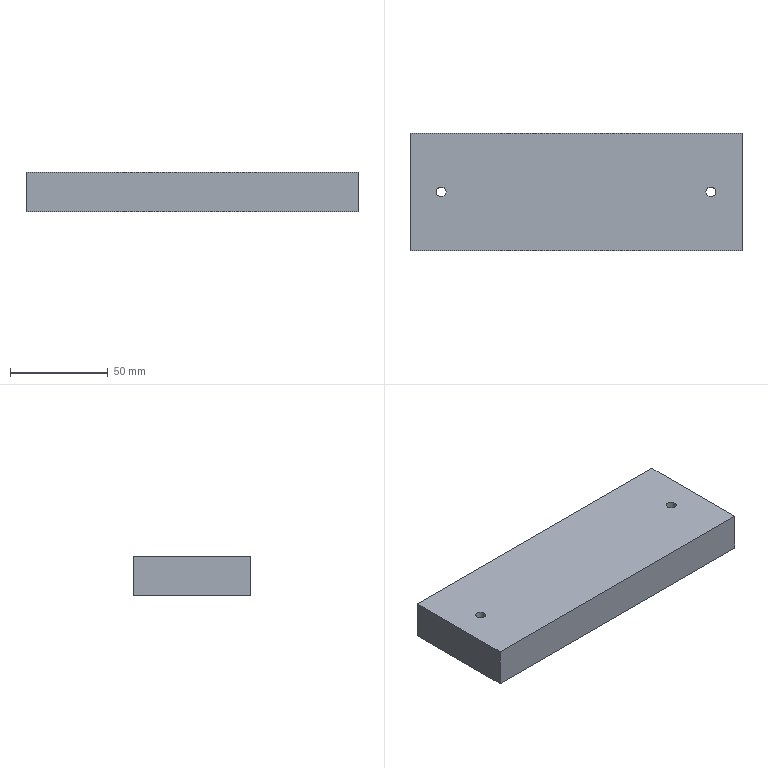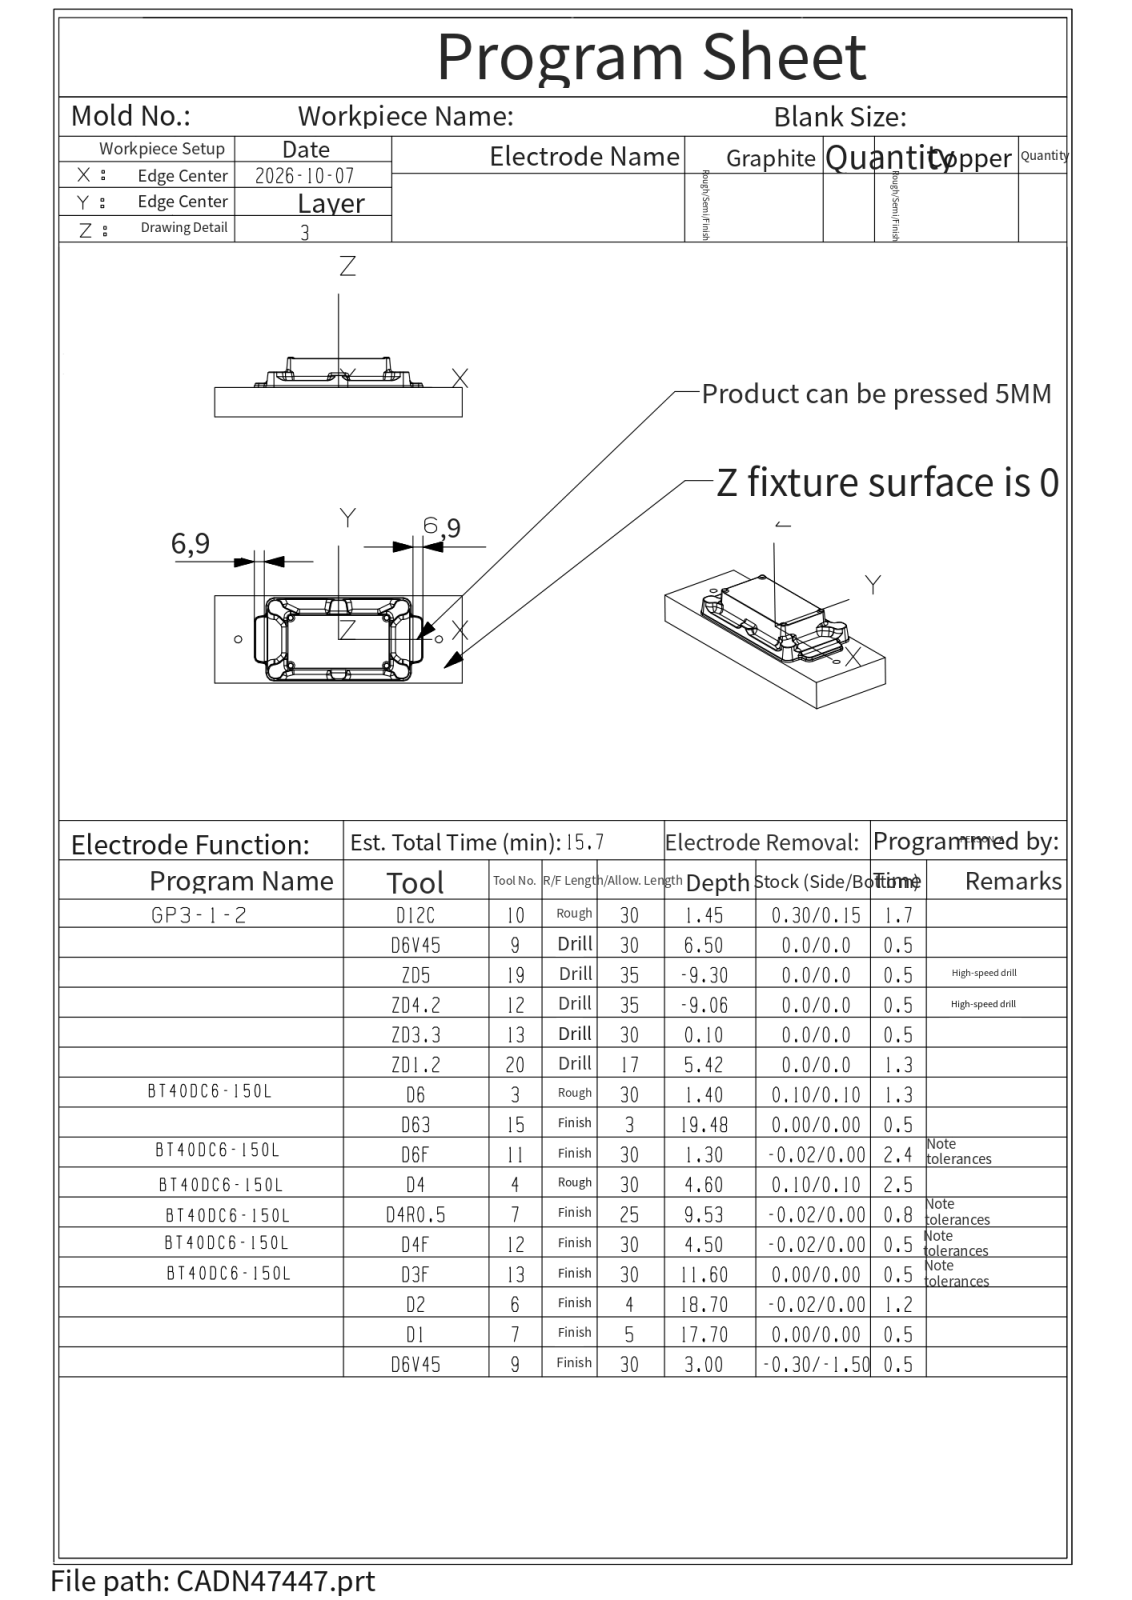NC program | NX | posted by the shop | part box 170 x 60 x 20 mm
Lines 1 to 1922 of 17682, first 1740 of 1922 lines:
%
O0001
G40 G49 G80 G90
G91 G28 Z0.0
N01
T10 M06
T02
( name=D12C    T=10 )
( XY = 0.30 )
( Z = 0.15 )
G00 G90 G54 X8.475 Y-8.751 S8000 M03
G43 Z27.98 H10 M08
Z23.088
G01 Z22.588 F4800.
X4.574 Y-7.625
G03 X-2.855 Y-11.725 I-1.664 J-5.765
G01 X-2.913 Y-11.927 F6000.
G02 X-3.047 Y-12.23 I-1.198 J.346
G01 X-3.202 Y-12.485
G02 X-3.859 Y-13.168 I-2.36 J1.613
X-5.449 Y-13.661 I-1.586 J2.307
X-6.373 Y-13.472 I.117 J2.913
X-7.504 Y-9.38 I.977 J2.472
X-5.57 Y-8.348 I2.111 J-1.627
X-3.795 Y-8.88 I.158 J-2.698
X-2.797 Y-11.523 I-1.611 J-2.118
G01 X-2.855 Y-11.725
G03 X1.245 Y-19.154 I5.765 J-1.664
G01 X5.151 Y-20.281
Z23.088
G00 Z24.48
G01 X-14.223 Y.1
G00 Z22.197
G01 Z21.697 F4800.
X-13.247 Y-3.888
G03 X-5.992 Y-8.29 I5.828 J1.427
G01 X-5.883 Y-8.263 F6000.
X-5.752 Y-8.242
G02 X-5.169 Y-8.23 I.336 J-2.119
G01 X-4.93 Y-8.259
G02 X-2.866 Y-9.849 I-.472 J-2.748
X-4.961 Y-13.746 I-2.535 J-1.149
G03 X-5. Y-13.752 I.783 J-5.343
G02 X-6.161 Y-13.673 I-.405 J2.627
X-6.231 Y-8.348 I.759 J2.673
G01 X-5.992 Y-8.29
G03 X-1.591 Y-1.035 I-1.427 J5.828
G01 X-2.552 Y2.892
Z22.197
G00 Z23.588
G01 X-.765 Y-24.536
G00 Z21.305
G01 Z20.805 F4800.
X-.344 Y-20.474
G03 X-5.694 Y-13.888 I-5.968 J.618
G02 X-5.99 Y-13.85 I.724 J6.99 F6000.
X-7.385 Y-13.126 I.656 J2.967
X-7.837 Y-12.591 I3.172 J3.134
X-8.116 Y-9.965 I2.485 J1.592
X-6.247 Y-8.222 I2.707 J-1.028
G01 X-5.889 Y-8.134
G02 X-5.763 Y-8.12 I.448 J-3.51
G03 X-5.58 Y-8.1 I-.49 J5.378
G02 X-5.206 Y-8.101 I.186 J-1.478
G03 X-4.966 Y-8.126 I.682 J5.357
G02 X-4.591 Y-8.202 I-.131 J-1.601
G01 X-4.414 Y-8.266
G02 X-2.77 Y-12.236 I-.983 J-2.732
G01 X-2.874 Y-12.432
G02 X-3.521 Y-13.21 I-2.185 J1.159
G01 X-3.75 Y-13.392
G02 X-5.396 Y-13.912 I-1.669 J2.415
X-5.694 Y-13.888 I.426 J7.014
G03 X-12.28 Y-19.237 I-.618 J-5.968
G01 X-12.701 Y-23.302
Z21.305
G00 Z22.697
G01 X-10.664 Y2.576
G00 Z20.413
G01 Z19.913 F4800.
X-10.84 Y-1.626
G03 X-5.095 Y-7.871 I5.995 J-.25
X-4.915 Y-7.876 I.225 J5.395 F6000.
G02 X-2.674 Y-9.426 I-.504 J-3.124
X-2.451 Y-9.876 I-3.54 J-2.03
G01 X-2.33 Y-10.244
G02 X-4.767 Y-14.098 I-3.096 J-.74
X-5.894 Y-14.116 I-.634 J4.409
X-7.484 Y-13.362 I.47 J3.046
G03 X-7.661 Y-13.21 I-3.61 J-4.016
G02 X-7.742 Y-13.125 I.3 J.365
G03 X-7.872 Y-12.955 I-4.352 J-3.196
G02 X-7.149 Y-8.381 I2.454 J1.956
G03 X-7.097 Y-8.346 I-2.979 J4.504
G02 X-5.275 Y-7.861 I1.606 J-2.369
G03 X-5.095 Y-7.871 I.406 J5.385
X1.15 Y-2.127 I.25 J5.995
G01 X1.319 Y1.912
Z20.413
G00 Z26.48
G01 X-10.16 Y-54.913
G00 Z23.088
G01 Z22.588 F4800.
X-12.553 Y-51.584
G03 X-20.927 Y-50.214 I-4.872 J-3.502
G01 X-20.942 Y-50.224 F6000.
G02 X-21.444 Y-50.482 I-2.494 J4.251
X-23.912 Y-50.19 I-.951 J2.541
X-24.882 Y-48.956 I1.656 J2.301
X-25.025 Y-47.576 I2.704 J.976
X-23.914 Y-45.817 I2.679 J-.461
X-22.772 Y-45.369 I1.543 J-2.25
X-19.812 Y-47.394 I.368 J-2.638
X-20.479 Y-49.842 I-2.629 J-.599
X-20.927 Y-50.214 I-2.888 J3.023
G03 X-22.297 Y-58.588 I3.502 J-4.872
G01 X-19.958 Y-61.842
Z23.088
G00 Z24.48
G01 X-17.109 Y-61.159
G00 Z22.197
G01 Z21.697 F4800.
X-16.891 Y-57.085
G03 X-22.561 Y-50.773 I-5.991 J.321
G01 X-22.581 Y-50.772 F6000.
G02 X-23.818 Y-50.39 I.13 J2.615
X-23.952 Y-45.693 I1.415 J2.39
X-20.129 Y-46.395 I1.553 J-2.301
X-20.207 Y-49.71 I-2.265 J-1.605
X-22.561 Y-50.773 I-2.176 J1.681
G03 X-28.874 Y-56.443 I-.321 J-5.991
G01 X-29.091 Y-60.502
Z22.197
G00 Z23.588
G01 X-13.922 Y-36.477
G00 Z21.305
G01 Z20.805 F4800.
X-17.484 Y-38.421
G03 X-19.876 Y-46.563 I2.875 J-5.266
X-19.817 Y-46.667 I4.74 J2.588 F6000.
G02 X-19.598 Y-47.23 I-1.742 J-1.002
G03 X-19.576 Y-47.323 I5.269 J1.181
G02 X-22.552 Y-50.899 I-2.816 J-.683
G03 X-22.613 Y-50.896 I-.298 J-5.392
G02 X-23.229 Y-50.783 I.101 J2.283
G03 X-23.352 Y-50.744 I-1.695 J-5.127
G02 X-23.465 Y-50.708 I.966 J3.173
G01 X-23.825 Y-50.53
G02 X-24.417 Y-45.908 I1.422 J2.531
G01 X-24.206 Y-45.725
G02 X-22.064 Y-45.116 I1.79 J-2.227
X-20.146 Y-46.17 I-.317 J-2.847
G03 X-20.033 Y-46.307 I4.212 J3.379
G02 X-19.932 Y-46.457 I-.593 J-.509
G03 X-19.876 Y-46.563 I4.796 J2.482
X-11.734 Y-48.954 I5.266 J2.875
G01 X-8.131 Y-46.987
Z21.305
G00 Z22.697
G01 X-32.017 Y-58.92
G00 Z20.413
G01 Z19.913 F4800.
X-28.284 Y-57.257
G03 X-25.246 Y-49.334 I-2.442 J5.481
G02 X-25.369 Y-49.033 I4.876 J2.173 F6000.
X-25.404 Y-47.068 I2.758 J1.033
G03 X-25.384 Y-47.005 I-5.122 J1.71
G02 X-24.867 Y-46.046 I2.836 J-.908
G03 X-24.769 Y-45.92 I-4.207 J3.386
G02 X-24.371 Y-45.541 I1.356 J-1.027
G01 X-24.157 Y-45.395
G02 X-22.384 Y-44.836 I1.816 J-2.666
X-21.74 Y-44.908 I-.935 J-11.234
X-20.262 Y-45.672 I-.782 J-3.326
X-19.264 Y-47.633 I-2.222 J-2.364
X-19.248 Y-48.216 I-5.497 J-.449
X-21.26 Y-50.949 I-3.181 J.234
X-23.097 Y-51.071 I-1.142 J3.317
X-25.104 Y-49.627 I.711 J3.105
X-25.246 Y-49.334 I4.735 J2.466
G03 X-33.168 Y-46.296 I-5.481 J-2.442
G01 X-36.956 Y-47.983
Z20.413
G00 Z26.48
G01 X-66.051 Y-60.544
G00 Z23.088
G01 Z22.588 F4800.
X-66.138 Y-56.513
G03 X-72.267 Y-50.645 I-5.999 J-.13
G01 X-72.487 Y-50.65 F6000.
X-72.684 Y-50.634
X-73.037 Y-50.577
G02 X-73.654 Y-50.338 I.508 J2.226
G03 X-73.82 Y-50.248 I-2.66 J-4.699
G02 X-73.931 Y-50.174 I.296 J.568
G03 X-74.046 Y-50.082 I-3.429 J-4.171
G02 X-74.953 Y-48.721 I1.585 J2.039
X-72.71 Y-45.364 I2.549 J.725
X-70.972 Y-45.759 I.316 J-2.63
G01 X-70.592 Y-46.055
G02 X-70.616 Y-49.969 I-1.808 J-1.945
G01 X-70.767 Y-50.094
G02 X-71.508 Y-50.501 I-1.484 J1.822
G01 X-71.655 Y-50.546
X-71.779 Y-50.581
X-71.996 Y-50.62
X-72.267 Y-50.645
G03 X-77.681 Y-57.179 I.56 J-5.974
G01 X-77.306 Y-61.173
Z23.088
G00 Z24.48
G01 X-60.214 Y-55.256
G00 Z22.197
G01 Z21.697 F4800.
X-62.5 Y-51.89
G03 X-70.834 Y-50.298 I-4.964 J-3.371
G01 X-70.841 Y-50.302 F6000.
G02 X-72.947 Y-50.726 I-1.554 J2.282
X-75.084 Y-48.727 I.546 J2.726
X-74.254 Y-45.927 I2.683 J.728
X-72.009 Y-45.245 I1.857 J-2.078
X-70.188 Y-49.687 I-.391 J-2.755
X-70.834 Y-50.298 I-2.166 J1.648
G03 X-72.427 Y-58.632 I3.371 J-4.964
G01 X-70.14 Y-62.
Z22.197
G00 Z23.588
G01 X-79.826 Y-35.774
G00 Z21.305
G01 Z20.805 F4800.
X-79.362 Y-39.834
G03 X-72.721 Y-45.115 I5.961 J.68
G01 X-72.714 Y-45.114 F6000.
G02 X-70.425 Y-45.868 I.329 J-2.851
X-69.597 Y-48.765 I-1.966 J-2.129
X-70.546 Y-50.234 I-2.793 J.764
X-71.339 Y-50.711 I-2.005 J2.436
X-73.46 Y-50.706 I-1.053 J2.767
X-75.282 Y-47.627 I1.057 J2.705
X-72.721 Y-45.115 I2.88 J-.374
G03 X-67.44 Y-38.473 I-.68 J5.961
G01 X-67.903 Y-34.417
Z21.305
G00 Z22.697
G01 X-86.311 Y-52.287
G00 Z20.413
G01 Z19.913 F4800.
X-82.22 Y-52.803
G03 X-75.516 Y-47.602 I.752 J5.953
G01 X-75.476 Y-47.286 F6000.
G02 X-73.328 Y-44.988 I3.08 J-.726
G01 X-73.173 Y-44.94
G02 X-72.603 Y-44.86 I.586 J-2.097
G03 X-72.464 Y-44.857 I-.039 J5.4
G02 X-70.723 Y-45.338 I.1 J-3.033
G03 X-70.601 Y-45.414 I2.922 J4.541
G02 X-70.018 Y-45.938 I-1.096 J-1.806
G03 X-69.879 Y-46.112 I4.292 J3.277
G02 X-69.478 Y-46.839 I-1.696 J-1.409
G03 X-69.411 Y-47.032 I5.135 J1.671
G02 X-69.259 Y-48.251 I-2.546 J-.936
G03 X-69.275 Y-48.428 I5.371 J-.563
G02 X-69.375 Y-48.873 I-1.524 J.109
G03 X-69.451 Y-49.081 I5.032 J-1.959
G02 X-71.027 Y-50.832 I-2.845 J.975
G03 X-71.097 Y-50.865 I2.278 J-4.896
G02 X-72.717 Y-51.139 I-1.284 J2.66
G03 X-72.832 Y-51.127 I-.616 J-5.365
G02 X-73.417 Y-50.987 I.197 J2.111
G03 X-73.528 Y-50.944 I-1.991 J-5.02
G02 X-75.115 Y-49.597 I1.061 J2.858
G03 X-75.142 Y-49.55 I-4.691 J-2.675
G02 X-75.556 Y-47.919 I2.634 J1.537
G01 X-75.516 Y-47.602
G03 X-80.717 Y-40.898 I-5.953 J.752
G01 X-84.802 Y-40.382
Z20.413
G00 Z26.48
G01 X-97.992 Y-22.123
G00 Z23.088
G01 Z22.588 F4800.
X-94.38 Y-20.287
G03 X-91.749 Y-12.22 I-2.719 J5.349
G01 X-91.87 Y-11.982 F6000.
G02 X-91.887 Y-10.06 I2.554 J.983
G01 X-91.734 Y-9.738
G02 X-89.231 Y-8.348 I2.338 J-1.261
X-87.165 Y-9.565 I-.176 J-2.661
X-86.816 Y-11.613 I-2.231 J-1.433
X-87.76 Y-13.088 I-2.575 J.609
X-88.677 Y-13.554 I-1.592 J2.
X-90.262 Y-13.511 I-.726 J2.488
X-91.619 Y-12.452 I.847 J2.485
G03 X-91.653 Y-12.4 I-4.535 J-2.931
G01 X-91.689 Y-12.339
X-91.749 Y-12.22
G03 X-99.817 Y-9.589 I-5.349 J-2.719
G01 X-103.446 Y-11.434
Z23.088
G00 Z24.48
G01 X-95.392 Y1.852
G00 Z22.197
G01 Z21.697 F4800.
Y-2.218
G03 X-89.392 Y-8.218 I6. J0.0
G02 X-89.227 Y-8.223 I0.0 J-2.797 F6000.
X-86.993 Y-9.606 I-.181 J-2.789
X-88.404 Y-13.596 I-2.406 J-1.394
X-89.819 Y-13.75 I-.994 J2.562
X-91.46 Y-9.131 I.422 J2.751
X-89.392 Y-8.218 I2.067 J-1.884
G03 X-83.392 Y-2.218 I0.0 J6.
G01 Y1.845
Z22.197
G00 Z23.588
G01 X-99.464 Y-.833
G00 Z21.305
G01 Z20.805 F4800.
X-98.052 Y-4.686
G03 X-90.354 Y-8.256 I5.634 J2.064
X-90.324 Y-8.245 I-1.858 J5.07 F6000.
G02 X-89.646 Y-8.104 I.798 J-2.139
G03 X-89.473 Y-8.092 I-.284 J5.393
G02 X-89.245 Y-8.097 I.092 J-1.086
G01 X-88.852 Y-8.149
X-88.551 Y-8.222
G02 X-86.828 Y-12.352 I-.844 J-2.776
G01 X-86.961 Y-12.59
G02 X-87.123 Y-12.803 I-1.97 J1.33
G03 X-87.178 Y-12.869 I4.108 J-3.505
G02 X-88.605 Y-13.794 I-2.182 J1.802
G03 X-88.772 Y-13.843 I1.441 J-5.204
G02 X-88.833 Y-13.856 I-.1 J.32
G03 X-88.995 Y-13.878 I.632 J-5.363
G02 X-89.826 I-.415 J2.792
X-91.63 Y-12.862 I.435 J2.883
X-90.384 Y-8.267 I2.228 J1.862
G03 X-90.354 Y-8.256 I-1.827 J5.081
X-86.784 Y-.558 I-2.064 J5.634
G01 X-88.181 Y3.254
Z21.305
G00 Z22.697
G01 X-90.208 Y-25.527
G00 Z20.413
G01 Z19.913 F4800.
X-88.313 Y-21.874
G03 X-90.876 Y-13.785 I-5.326 J2.763
G02 X-91.167 Y-13.626 I3.238 J6.241 F6000.
X-92.306 Y-12.227 I2.002 J2.794
X-92.552 Y-11.147 I4.098 J1.499
X-92.116 Y-9.388 I3.422 J.086
X-91.125 Y-8.344 I3.026 J-1.88
X-89.708 Y-7.867 I1.754 J-2.868
G03 X-89.462 Y-7.837 I-.54 J5.373
G02 X-89.314 I.074 J-.504
G03 X-89.056 Y-7.868 I.786 J5.343
G02 X-87.341 Y-8.615 I-.297 J-3.024
G03 X-87.31 Y-8.642 I3.575 J4.047
G02 X-86.307 Y-11.595 I-2.034 J-2.338
G01 X-86.406 Y-11.966
X-86.51 Y-12.264
X-86.617 Y-12.47
G02 X-88.991 Y-14.123 I-2.745 J1.411
G01 X-89.427 Y-14.149
G02 X-90.578 Y-13.931 I.016 J3.24
X-90.876 Y-13.785 I2.939 J6.387
G03 X-98.965 Y-16.348 I-2.763 J-5.326
G01 X-100.848 Y-19.978
Z20.413
G00 Z21.805
G01 X-53.396 Y14.562
G00 Z19.522
G01 Z19.022 F4800.
Y9.162
G03 X-47.396 Y3.162 I6. J0.0
G01 X-3.106 F6000.
G02 X-2.884 Y3.148 I0.0 J-1.709
G01 X-1.478 Y2.964
G02 X-1.264 Y2.902 I-.163 J-.955
G03 X-1.236 Y2.89 I2.1 J4.975
G01 X-.136 Y2.433
G02 X.279 Y2.193 I-.709 J-1.707
G01 X1.161 Y1.517
G03 X1.224 Y1.469 I3.285 J4.286
G02 X1.36 Y1.341 I-.474 J-.638
X2.325 Y.089 I-15.618 J-13.034
X2.497 Y-.287 I-2.928 J-1.57
G03 X2.597 Y-.528 I5.039 J1.941
G02 X2.96 Y-1.442 I-12.011 J-5.306
X2.972 Y-1.49 I-.218 J-.077
G01 X3.153 Y-2.931
G02 X3.163 Y-4.148 I-25.914 J-.825
G03 X7.354 Y-9.493 I5.399 J-.082
G02 X8.809 Y-9.941 I-2.323 J-10.116
X9.272 Y-10.229 I-1.927 J-3.619
G03 X9.469 Y-10.364 I3.147 J4.388
G02 X9.862 Y-10.673 I-1.527 J-2.342
G01 X10.05 Y-10.888
G03 X10.085 Y-10.928 I4.065 J3.555
G02 X10.548 Y-11.517 I-4.507 J-4.02
X10.999 Y-12.55 I-7.38 J-3.839
X11.043 Y-12.757 I-1.009 J-.322
G03 X11.098 Y-13.14 I5.368 J.584
G02 X11.164 Y-13.863 I-3.973 J-.723
G01 X11.165 Y-38.105
G02 X11.097 Y-38.868 I-4.291 J0.0
G03 X11.043 Y-39.24 I5.314 J-.959
G02 X10.998 Y-39.453 I-1.075 J.118
X10.553 Y-40.471 I-7.566 J2.698
X9.895 Y-41.294 I-6.973 J4.9
X9.471 Y-41.635 I-1.938 J1.983
G03 X9.281 Y-41.764 I2.948 J-4.524
G02 X8.802 Y-42.061 I-2.529 J3.543
X7.364 Y-42.503 I-3.68 J9.414
G03 X3.162 Y-47.857 I1.198 J-5.266
G02 X3.153 Y-49.071 I-25.532 J-.418
G01 X2.971 Y-50.513
G02 X2.962 Y-50.552 I-.178 J.022
X2.586 Y-51.495 I-14.673 J5.291
G03 X2.497 Y-51.714 I4.95 J-2.159
G02 X2.324 Y-52.091 I-3.076 J1.184
X1.364 Y-53.336 I-15.824 J11.205
X1.225 Y-53.469 I-.604 J.494
G03 X1.163 Y-53.516 I3.222 J-4.334
G01 X.304 Y-54.174
G02 X-.449 Y-54.569 I-1.75 J2.418
G03 X-.895 Y-54.749 I1.803 J-5.09
G02 X-1.386 Y-54.94 I-1.815 J3.962
X-1.975 Y-55.031 I-1.216 J5.884
G03 X-2.327 Y-55.08 I.563 J-5.371
G02 X-3.285 Y-55.162 I-.958 J5.57
G01 X-91.695
G02 X-91.933 Y-55.146 I0.0 J1.82
G01 X-93.321 Y-54.963
G02 X-93.563 Y-54.889 I.157 J.951
G01 X-94.658 Y-54.435
G02 X-95.077 Y-54.192 I.715 J1.722
G01 X-95.957 Y-53.517
G03 X-96.028 Y-53.464 I-3.286 J-4.285
G02 X-96.159 Y-53.34 I.455 J.613
X-97.088 Y-52.138 I15.84 J13.192
G01 X-97.173 Y-51.98
X-97.382 Y-51.5
G03 X-97.413 Y-51.43 I-4.954 J-2.15
G01 X-97.719 Y-50.683
G02 X-97.761 Y-50.527 I.611 J.25
X-97.95 Y-49.095 I54.72 J7.95
X-97.963 Y-47.839 I27.766 J.901
G03 X-102.154 Y-42.507 I-5.4 J.069
G02 X-103.603 Y-42.06 I2.315 J10.088
X-104.084 Y-41.762 I2.075 J3.883
G03 X-104.268 Y-41.637 I-3.135 J-4.397
G02 X-104.697 Y-41.292 I1.527 J2.341
X-105.354 Y-40.469 I6.077 J5.527
X-105.798 Y-39.45 I7.563 J3.899
X-105.843 Y-39.237 I1.057 J.335
G03 X-105.898 Y-38.858 I-5.368 J-.59
G02 X-105.963 Y-38.156 I3.895 J.71
G01 Y-37.748
Y-14.252
Y-13.844
G02 X-105.898 Y-13.142 I3.959 J-.008
G03 X-105.839 Y-12.729 I-5.312 J.969
G02 X-105.798 Y-12.55 I.754 J-.078
X-105.356 Y-11.533 I8.137 J-2.94
X-104.695 Y-10.705 I7.015 J-4.919
X-104.268 Y-10.363 I1.969 J-2.02
G03 X-104.079 Y-10.234 I-2.951 J4.522
G02 X-103.593 Y-9.933 I2.501 J-3.5
X-102.214 Y-9.513 I3.252 J-8.197
G03 X-97.96 Y-4.176 I-1.147 J5.277
G02 X-97.949 Y-2.894 I32.068 J.356
X-97.76 Y-1.467 I53.843 J-6.385
X-97.723 Y-1.329 I.583 J-.085
G01 X-97.401 Y-.544
G03 X-97.382 Y-.5 I-4.933 J2.198
G01 X-97.173 Y-.019
X-97.087 Y.139
G02 X-96.142 Y1.361 I16.773 J-11.994
X-96.103 Y1.399 I.212 J-.177
G01 X-95.573 Y1.823
G02 X-94.823 Y2.354 I4.808 J-6.005
X-94.299 Y2.589 I1.916 J-3.571
G03 X-93.926 Y2.741 I-1.855 J5.072
G02 X-93.396 Y2.945 I2.012 J-4.441
X-92.827 Y3.034 I1.149 J-5.462
G03 X-92.497 Y3.079 I-.561 J5.371
G02 X-91.496 Y3.162 I1.001 J-5.983
G01 X-47.396
Y-5.838
X-5.747
G03 X2.164 Y-17.13 I14.31 J1.608
G01 X2.165 Y-34.867
G03 X-5.749 Y-46.162 I6.396 J-12.901
G01 X-89.052
G03 X-96.963 Y-34.87 I-14.31 J-1.609
G01 Y-17.137
G03 X-89.049 Y-5.838 I-6.397 J12.901
G01 X-47.396
Y-14.838
X-12.295
G03 X-6.836 Y-21.849 I20.857 J10.608
G01 X-6.835 Y-30.147
G03 X-12.297 Y-37.162 I15.397 J-17.621
G01 X-82.505
G03 X-87.963 Y-30.151 I-20.857 J-10.609
G01 Y-21.857
G03 X-82.499 Y-14.838 I-15.397 J17.621
G01 X-47.396
Y-23.838
X-17.23
G03 X-15.836 Y-25.548 I25.793 J19.608
G01 Y-26.448
G03 X-17.233 Y-28.162 I24.397 J-21.32
G01 X-77.569
G03 X-78.963 Y-26.452 I-25.793 J-19.609
G01 Y-25.557
G03 X-77.562 Y-23.838 I-24.397 J21.32
G01 X-47.396
G03 X-41.396 Y-17.838 I0.0 J6.
G01 Z19.522
G00 Z20.913
G01 X-53.396 Y14.565
G00 Z18.63
G01 Z18.13 F4800.
Y9.165
G03 X-47.396 Y3.165 I6. J0.0
G01 X-3.303 F6000.
G02 X-2.304 Y3.082 I0.0 J-6.051
G03 X-1.969 Y3.036 I.892 J5.326
G02 X-1.437 Y2.954 I-.565 J-5.444
X-.03 Y2.387 I-3.532 J-10.78
X.232 Y2.229 I-.723 J-1.496
X1.278 Y1.424 I-18.238 J-24.777
X1.551 Y1.118 I-1.978 J-2.045
G03 X1.585 Y1.075 I4.274 J3.301
G02 X2.323 Y.095 I-21.59 J-17.03
X2.498 Y-.283 I-2.689 J-1.478
G03 X2.587 Y-.499 I5.041 J1.937
G02 X2.951 Y-1.411 I-14.812 J-6.439
X2.978 Y-1.522 I-.479 J-.174
G01 X3.155 Y-2.924
G02 X3.164 Y-4.156 I-28.651 J-.843
G03 X7.362 Y-9.493 I5.4 J-.073
G02 X8.802 Y-9.936 I-2.269 J-9.939
X9.279 Y-10.232 I-2.044 J-3.823
G03 X9.469 Y-10.362 I3.14 J4.393
G02 X9.895 Y-10.703 I-1.546 J-2.37
X10.553 Y-11.527 I-6.479 J-5.85
X11.002 Y-12.552 I-7.419 J-3.856
X11.044 Y-12.755 I-1.001 J-.317
G03 X11.091 Y-13.089 I5.369 J.582
G02 X11.164 Y-13.708 I-5.833 J-1.004
G01 X11.165 Y-14.252
Y-37.748
X11.164 Y-38.292
G02 X11.091 Y-38.911 I-5.906 J.384
G03 X11.045 Y-39.236 I5.322 J-.916
G02 X11. Y-39.452 I-1.107 J.122
X10.543 Y-40.493 I-7.763 J2.783
X10.086 Y-41.072 I-5.001 J3.473
G03 X10.057 Y-41.105 I4.03 J-3.594
G01 X9.864 Y-41.325
G02 X9.473 Y-41.633 I-1.899 J2.008
G03 X9.277 Y-41.767 I2.946 J-4.526
G02 X8.803 Y-42.062 I-2.51 J3.508
X7.362 Y-42.504 I-3.707 J9.5
G03 X3.163 Y-47.846 I1.2 J-5.265
G02 X3.154 Y-49.08 I-29.116 J-.416
G01 X2.983 Y-50.437
G02 X2.906 Y-50.725 I-1.116 J.141
G01 X2.445 Y-51.843
G02 X2.324 Y-52.094 I-2.338 J.966
X1.354 Y-53.349 I-17.801 J12.762
X1.231 Y-53.466 I-.548 J.456
G03 X1.165 Y-53.515 I3.218 J-4.337
G01 X.303 Y-54.175
G02 X-.443 Y-54.567 I-1.72 J2.369
G03 X-.901 Y-54.753 I1.797 J-5.092
G02 X-1.359 Y-54.932 I-1.782 J3.876
X-3.011 Y-55.158 I-2.699 J13.584
G01 X-3.513 Y-55.163
X-91.681
G02 X-91.979 Y-55.143 I0.0 J2.245
G01 X-93.327 Y-54.963
G02 X-93.526 Y-54.905 I.135 J.844
G03 X-93.567 Y-54.888 I-2.109 J-4.971
G01 X-94.746 Y-54.399
X-94.766 Y-54.389
G02 X-95.794 Y-53.649 I4.846 J7.809
G03 X-95.869 Y-53.588 I-3.451 J-4.153
G01 X-96.11 Y-53.394
G02 X-96.137 Y-53.368 I.116 J.145
X-97.084 Y-52.146 I16.91 J14.084
G01 X-97.183 Y-51.964
G02 X-97.733 Y-50.644 I35.401 J15.539
X-97.758 Y-50.551 I.389 J.154
X-97.951 Y-49.098 I55.21 J8.067
X-97.963 Y-47.835 I29.527 J.908
G03 X-102.16 Y-42.506 I-5.4 J.065
G02 X-103.602 Y-42.062 I2.279 J9.974
X-104.086 Y-41.762 I2.1 J3.929
G03 X-104.266 Y-41.639 I-3.133 J-4.398
G02 X-104.696 Y-41.294 I1.546 J2.367
X-105.354 Y-40.471 I6.311 J5.72
X-105.796 Y-39.458 I7.005 J3.655
X-105.845 Y-39.226 I1.135 J.365
G03 X-105.899 Y-38.858 I-5.366 J-.601
G02 X-105.964 Y-38.156 I3.895 J.71
G01 Y-37.748
Y-14.252
Y-13.844
G02 X-105.899 Y-13.142 I3.959 J-.008
G03 X-105.84 Y-12.728 I-5.312 J.969
G02 X-105.8 Y-12.551 I.74 J-.076
X-105.344 Y-11.51 I8.246 J-2.989
X-104.888 Y-10.93 I4.913 J-3.4
G03 X-104.682 Y-10.685 I-4.028 J3.597
G02 X-103.553 Y-9.913 I4.143 J-4.846
X-103.075 Y-9.749 I2.039 J-5.141
G03 X-102.84 Y-9.674 I-1.524 J5.181
G02 X-102.322 Y-9.534 I1.265 J-3.671
G03 X-97.962 Y-4.167 I-1.039 J5.299
G02 X-97.951 Y-2.897 I29.632 J.377
X-97.757 Y-1.44 I50.83 J-6.007
X-97.734 Y-1.357 I.355 J-.052
G01 X-97.404 Y-.551
G03 X-97.379 Y-.494 I-4.929 J2.205
G01 X-97.172 Y-.017
X-97.092 Y.131
G02 X-96.382 Y1.075 I21.404 J-15.383
G03 X-96.342 Y1.125 I-4.239 J3.345
G02 X-96.086 Y1.414 I2.193 J-1.688
X-95.142 Y2.145 I28.862 J-36.323
X-94.343 Y2.575 I1.805 J-2.395
G03 X-93.902 Y2.754 I-1.811 J5.087
G02 X-93.41 Y2.944 I1.765 J-3.846
X-92.824 Y3.036 I1.188 J-5.645
G03 X-92.496 Y3.081 I-.564 J5.37
G02 X-91.485 Y3.165 I1.011 J-6.041
G01 X-47.396
Y-5.835
X-5.746
G03 X2.165 Y-17.129 I14.31 J1.607
G01 Y-34.868
G03 X-5.748 Y-46.163 I6.397 J-12.901
G01 X-89.052
G03 X-96.964 Y-34.87 I-14.31 J-1.607
G01 Y-17.136
G03 X-89.05 Y-5.835 I-6.397 J12.901
G01 X-47.396
Y-14.835
X-12.294
G03 X-6.835 Y-21.848 I20.858 J10.607
G01 Y-30.148
G03 X-12.296 Y-37.163 I15.397 J-17.621
G01 X-82.505
G03 X-87.964 Y-30.15 I-20.858 J-10.607
G01 Y-21.856
G03 X-82.5 Y-14.835 I-15.397 J17.621
G01 X-47.396
Y-23.835
X-17.23
G03 X-15.835 Y-25.547 I25.794 J19.607
G01 Y-26.449
G03 X-17.232 Y-28.163 I24.397 J-21.32
G01 X-77.569
G03 X-78.964 Y-26.451 I-25.794 J-19.607
G01 Y-25.556
G03 X-77.562 Y-23.835 I-24.397 J21.32
G01 X-47.396
G03 X-41.396 Y-17.835 I0.0 J6.
G01 Z18.63
G00 Z27.98
G00 X-51.101 Y-19.768 S8000 M03
M08
Z18.18
G01 X-51.686 Y-20.398 Z18.15 F4800.
X-52.155 Y-21.119 Z18.12
X-52.503 Y-21.905 Z18.09
X-52.723 Y-22.736 Z18.06
X-52.809 Y-23.591 Z18.03
X-52.758 Y-24.449 Z18.
X-52.571 Y-25.289 Z17.97
X-52.254 Y-26.088 Z17.94
X-51.815 Y-26.827 Z17.91
X-51.264 Y-27.487 Z17.88
X-50.615 Y-28.051 Z17.85
X-49.885 Y-28.505 Z17.82
X-49.092 Y-28.838 Z17.79
X-48.257 Y-29.042 Z17.76
X-47.4 Y-29.1 Z17.73
X-25.3 F6000.
Y-22.9
X-69.5
Y-29.1
X-47.4
Y-38.1
X-16.3
Y-13.9
X-78.5
Y-38.1
X-47.4
G03 X-41.4 Y-32.1 I0.0 J6.
G01 Z18.23
G00 Z27.98
M05
M09
G91 G28 Z0.0
M01
N02
T02 M06
T15
( name=D8    T=2 )
( XY = 0.30 )
( Z = 0.15 )
G00 G90 G54 X-18.616 Y-38.5 S10000 M03
G43 Z27.98 H02 M08
Z17.73
G03 X-17.016 Y-40.1 I1.6 J0.0 F4000.
G01 X-14.3 F5000.
Y-37.384
G03 X-15.9 Y-35.784 I-1.6 J0.0
G00 Z27.98
Y-16.216
Z17.73
G03 X-14.3 Y-14.616 I0.0 J1.6 F4000.
G01 Y-11.9 F5000.
X-17.016
G03 X-18.616 Y-13.5 I0.0 J-1.6
G00 Z27.98
X-76.184
Z17.73
G03 X-77.784 Y-11.9 I-1.6 J0.0 F4000.
G01 X-80.5 F5000.
Y-14.616
G03 X-78.9 Y-16.216 I1.6 J0.0
G00 Z27.98
Y-35.784
Z17.73
G03 X-80.5 Y-37.384 I0.0 J-1.6 F4000.
G01 Y-40.099 F5000.
X-80.499 Y-40.1
X-77.784
G03 X-76.184 Y-38.5 I0.0 J1.6
G00 Z27.98
G00 X-64.284 Y-25.6 S10000 M03
M08
Z17.78
G01 X-74.3 Z17.605 F4800.
Y-30.4 Z17.521
X-64.899 Z17.357
X-56.367 F6000.
X-56.235 Y-30.403
X-55.5 Y-30.442
Y-25.52
G02 X-56.4 Y-25.6 I-.9 J5.02
G01 X-74.3
Y-30.4
X-64.899
X-56.65 Z17.213
X-56.306 Y-30.401 Z17.207
X-55.962 Y-30.414 Z17.201
X-55.5 Y-30.432 Z17.193
Y-30.218 Z17.189
Y-26.093 Z17.117
Y-25.529 Z17.107
X-55.613 Y-25.539 Z17.105
X-55.954 Y-25.581 Z17.099
X-56.297 Y-25.599 Z17.093
X-56.641 Y-25.6 Z17.087
X-56.984 Z17.081
X-58.359 Z17.057
X-74.3
Y-30.4
X-64.899
X-56.65 Z16.913
X-56.306 Y-30.401 Z16.907
X-55.962 Y-30.41 Z16.901
X-55.5 Y-30.422 Z16.893
Y-30.217 Z16.889
Y-26.092 Z16.817
Y-25.529 Z16.807
X-55.614 Y-25.539 Z16.805
X-55.955 Y-25.581 Z16.799
X-56.298 Y-25.599 Z16.793
X-56.642 Y-25.6 Z16.787
X-56.986 Z16.781
X-58.361 Z16.757
X-74.3
Y-30.4
X-64.899
X-56.65 Z16.613
X-56.306 Y-30.401 Z16.607
X-55.962 Y-30.405 Z16.601
X-55.5 Y-30.411 Z16.593
Y-30.216 Z16.589
Y-26.091 Z16.517
Y-25.53 Z16.507
X-55.615 Y-25.54 Z16.505
X-55.957 Y-25.581 Z16.499
X-56.3 Y-25.599 Z16.493
X-56.644 Y-25.6 Z16.487
X-56.987 Z16.481
X-58.362 Z16.457
X-74.3
Y-30.4
X-64.899
X-56.65 Z16.313
X-56.306 Y-30.403 Z16.307
X-55.962 Y-30.401 Z16.301
X-55.5 Y-30.4 Z16.293
Y-30.215 Z16.289
Y-26.09 Z16.217
Y-25.53 Z16.207
X-55.617 Y-25.54 Z16.205
X-55.958 Y-25.581 Z16.199
X-56.301 Y-25.599 Z16.193
X-56.645 Y-25.6 Z16.187
X-56.989 Z16.181
X-58.364 Z16.157
X-74.3
Y-30.4
X-64.899
X-56.65 Z16.013
X-56.306 Y-30.401 Z16.007
X-55.962 Z16.001
X-55.5 Z15.993
Y-30.203 Z15.989
Y-26.078 Z15.917
Y-25.531 Z15.908
X-55.629 Y-25.542 Z15.905
X-55.971 Y-25.582 Z15.899
X-56.314 Y-25.599 Z15.893
X-56.658 Y-25.6 Z15.887
X-57.689 Z15.869
X-58.376 Z15.857
X-74.3
Y-30.4
X-64.899
X-56.65 Z15.713
X-56.306 Y-30.401 Z15.707
X-55.962 Z15.701
X-55.5 Z15.693
Y-30.189 Z15.689
Y-26.064 Z15.617
Y-25.533 Z15.608
X-55.644 Y-25.544 Z15.605
X-55.985 Y-25.584 Z15.599
X-56.328 Y-25.599 Z15.593
X-56.672 Y-25.6 Z15.587
X-58.391 Z15.557
X-74.3
Y-30.4
X-64.899
X-56.65 Z15.413
X-56.306 Y-30.401 Z15.407
X-55.962 Z15.401
X-55.5 Z15.393
Y-30.179 Z15.389
Y-26.054 Z15.317
Y-25.535 Z15.308
X-55.655 Y-25.547 Z15.305
X-55.997 Y-25.585 Z15.299
X-56.34 Y-25.6 Z15.293
X-56.684 Z15.287
X-58.403 Z15.257
X-74.3
Y-30.4
X-64.899
X-56.65 Z15.113
X-56.306 Y-30.401 Z15.107
X-55.962 Z15.101
X-55.5 Z15.093
Y-30.175 Z15.089
Y-26.05 Z15.017
Y-25.545 Z15.008
X-55.659 Y-25.555 Z15.005
X-56.001 Y-25.587 Z14.999
X-56.345 Y-25.6 Z14.993
X-56.688 Z14.987
X-58.407 Z14.957
X-74.3
Y-30.4
X-64.899
X-56.65 Z14.813
X-56.306 Y-30.401 Z14.807
X-55.962 Z14.801
X-55.5 Z14.793
Y-30.175 Z14.789
Y-26.05 Z14.717
Y-25.556 Z14.708
X-55.661 Y-25.564 Z14.705
X-56.004 Y-25.591 Z14.699
X-56.348 Y-25.6 Z14.693
X-56.692 Z14.687
X-58.411 Z14.657
X-74.3
Y-30.4
X-64.899
X-56.65 Z14.513
X-56.306 Z14.507
X-55.962 Y-30.401 Z14.501
X-55.5 Z14.493
Y-30.175 Z14.489
Y-26.05 Z14.417
Y-25.567 Z14.408
X-55.673 Y-25.573 Z14.405
X-56.016 Y-25.595 Z14.399
X-56.36 Y-25.6 Z14.393
X-56.703 Z14.387
X-58.422 Z14.357
X-74.3
Y-30.4
X-64.899
X-56.65 Z14.213
X-56.306 Z14.207
X-55.962 Y-30.401 Z14.201
X-55.5 Z14.193
Y-30.175 Z14.189
Y-26.05 Z14.117
Y-25.578 Z14.109
X-55.686 Y-25.582 Z14.105
X-56.029 Y-25.597 Z14.099
X-56.373 Y-25.6 Z14.093
X-56.717 Z14.087
X-58.436 Z14.057
X-74.3
Y-30.4
X-64.899
X-56.65 Z13.913
X-56.306 Z13.907
X-55.962 Y-30.401 Z13.901
X-55.5 Z13.893
Y-30.175 Z13.889
Y-26.05 Z13.817
X-55.501 Y-25.589 Z13.809
X-55.7 Y-25.591 Z13.805
X-56.044 Y-25.598 Z13.799
X-56.388 Y-25.6 Z13.793
X-56.732 Z13.787
X-58.45 Z13.757
X-74.3
Y-30.4
X-64.899
X-56.65 Z13.613
X-56.306 Z13.607
X-55.962 Z13.601
X-55.5 Y-30.401 Z13.593
Y-30.175 Z13.589
Y-26.05 Z13.517
X-55.501 Y-25.597 Z13.509
X-55.715 Z13.505
X-56.059 Z13.499
X-56.403 Y-25.6 Z13.493
X-58.465 Z13.457
X-74.3
Y-30.4
X-64.899
X-56.65 Z13.313
X-56.306 Z13.307
X-55.962 Z13.301
X-55.5 Y-30.401 Z13.293
Y-30.175 Z13.289
Y-26.05 Z13.217
X-55.502 Y-25.599 Z13.209
X-55.731 Y-25.598 Z13.205
X-56.074 Z13.199
X-56.418 Y-25.6 Z13.193
X-58.48 Z13.157
X-74.3
Y-30.4
X-64.899
X-56.65 Z13.013
X-56.306 Z13.007
X-55.962 Z13.001
X-55.5 Y-30.401 Z12.993
Y-30.175 Z12.989
Y-26.05 Z12.917
X-55.502 Y-25.599 Z12.909
X-55.732 Y-25.598 Z12.905
X-56.076 Z12.899
X-56.42 Y-25.6 Z12.893
X-58.482 Z12.857
X-74.3
Y-30.4
X-64.899
X-56.65 Z12.713
X-56.306 Z12.707
X-55.962 Z12.701
X-55.5 Y-30.401 Z12.693
Y-30.175 Z12.689
Y-26.05 Z12.617
X-55.502 Y-25.599 Z12.609
X-55.732 Y-25.598 Z12.605
X-56.076 Z12.599
X-56.42 Y-25.6 Z12.593
X-58.482 Z12.557
X-74.3
Y-30.4
X-64.899
X-56.65 Z12.413
X-56.306 Z12.407
X-55.962 Z12.401
X-55.5 Y-30.401 Z12.393
Y-30.175 Z12.389
Y-26.05 Z12.317
X-55.502 Y-25.6 Z12.309
X-55.733 Y-25.598 Z12.305
X-56.076 Z12.299
X-56.42 Y-25.6 Z12.293
X-58.483 Z12.257
X-74.3
Y-30.4
X-64.899
X-56.65 Z12.113
X-56.306 Z12.107
X-55.962 Z12.101
X-55.5 Y-30.401 Z12.093
Y-30.175 Z12.089
Y-26.05 Z12.017
X-55.501 Y-25.599 Z12.009
X-55.733 Y-25.598 Z12.005
X-56.077 Z11.999
X-56.42 Y-25.6 Z11.993
X-58.483 Z11.957
X-74.3
Y-30.4
X-64.899
X-56.65 Z11.813
X-56.306 Z11.807
X-55.962 Z11.801
X-55.501 Z11.793
X-55.5 Y-30.175 Z11.789
Y-26.05 Z11.717
X-55.501 Y-25.599 Z11.709
X-55.733 Y-25.598 Z11.705
X-56.077 Z11.699
X-56.42 Y-25.6 Z11.693
X-58.483 Z11.657
X-74.3
Y-30.4
X-64.899
X-56.65 Z11.513
X-56.306 Z11.507
X-55.962 Z11.501
X-55.501 Z11.493
X-55.5 Y-30.175 Z11.489
Y-26.05 Z11.417
X-55.502 Y-25.6 Z11.409
X-55.733 Y-25.598 Z11.405
X-56.077 Z11.399
X-56.421 Y-25.6 Z11.393
X-58.483 Z11.357
X-74.3
Y-30.4
X-64.899
X-56.65 Z11.213
X-56.306 Z11.207
X-55.962 Z11.201
X-55.501 Z11.193
X-55.5 Y-30.175 Z11.189
Y-26.05 Z11.117
X-55.502 Y-25.6 Z11.109
X-55.733 Y-25.598 Z11.105
X-56.077 Z11.099
X-56.421 Y-25.6 Z11.093
X-58.483 Z11.057
X-74.3
Y-30.4
X-64.899
X-56.65 Z10.913
X-56.306 Y-30.399 Z10.907
X-55.962 Y-30.4 Z10.901
X-55.501 Z10.893
X-55.5 Y-30.175 Z10.889
Y-26.05 Z10.817
X-55.503 Y-25.6 Z10.809
X-55.734 Y-25.598 Z10.805
X-56.077 Y-25.599 Z10.799
X-56.421 Y-25.6 Z10.793
X-58.483 Z10.757
X-74.3
Y-30.4
X-64.899
X-56.65 Z10.613
X-56.306 Y-30.399 Z10.607
X-55.962 Y-30.4 Z10.601
X-55.501 Z10.593
X-55.5 Y-30.175 Z10.589
Y-26.05 Z10.517
X-55.502 Y-25.6 Z10.509
X-55.734 Y-25.598 Z10.505
X-56.077 Y-25.599 Z10.499
X-56.421 Y-25.6 Z10.493
X-58.484 Z10.457
X-74.3
Y-30.4
X-64.899
X-56.65 Z10.313
X-56.306 Y-30.399 Z10.307
X-55.962 Y-30.4 Z10.301
X-55.501 Z10.293
X-55.5 Y-30.175 Z10.289
Y-26.05 Z10.217
X-55.502 Y-25.6 Z10.209
X-55.734 Y-25.598 Z10.205
X-56.078 Y-25.599 Z10.199
X-56.421 Y-25.6 Z10.193
X-58.484 Z10.157
X-74.3
Y-30.4
X-64.899
X-56.65 Z10.013
X-56.306 Y-30.399 Z10.007
X-55.962 Y-30.4 Z10.001
X-55.501 Z9.993
X-55.5 Y-30.175 Z9.989
Y-26.05 Z9.917
X-55.502 Y-25.599 Z9.909
X-55.734 Y-25.598 Z9.905
X-56.078 Y-25.599 Z9.899
X-56.422 Y-25.6 Z9.893
X-58.484 Z9.857
X-74.3
Y-30.4
X-64.899
X-56.65 Z9.713
X-56.306 Y-30.399 Z9.707
X-55.962 Y-30.4 Z9.701
X-55.501 Z9.693
X-55.5 Y-30.175 Z9.689
Y-26.05 Z9.617
X-55.502 Y-25.599 Z9.609
X-55.734 Y-25.598 Z9.605
X-56.078 Y-25.599 Z9.599
X-56.422 Y-25.6 Z9.593
X-58.484 Z9.557
X-74.3
Y-30.4
X-64.899
X-56.65 Z9.413
X-56.306 Y-30.399 Z9.407
X-55.962 Y-30.4 Z9.401
X-55.501 Z9.393
X-55.5 Y-30.175 Z9.389
Y-26.05 Z9.317
X-55.502 Y-25.6 Z9.309
X-55.734 Y-25.598 Z9.305
X-56.078 Y-25.599 Z9.299
X-56.422 Y-25.6 Z9.293
X-58.484 Z9.257
X-74.3
Y-30.4
X-64.899
X-56.65 Z9.113
X-56.306 Y-30.399 Z9.107
X-55.962 Y-30.4 Z9.101
X-55.501 Z9.093
X-55.5 Y-30.175 Z9.089
Y-26.05 Z9.017
X-55.502 Y-25.6 Z9.009
X-55.735 Y-25.599 Z9.005
X-56.078 Z8.999
X-56.422 Y-25.6 Z8.993
X-58.484 Z8.957
X-74.3
Y-30.4
X-64.899
X-56.65 Z8.813
X-56.306 Y-30.401 Z8.807
X-55.962 Y-30.4 Z8.801
X-55.5 Y-30.398 Z8.793
Y-30.175 Z8.789
Y-26.05 Z8.717
X-55.502 Y-25.6 Z8.709
X-55.735 Y-25.599 Z8.705
X-56.078 Z8.699
X-56.422 Y-25.6 Z8.693
X-58.485 Z8.657
X-74.3
Y-30.4
X-64.899
X-56.65 Z8.513
X-56.306 Y-30.401 Z8.507
X-55.962 Y-30.4 Z8.501
X-55.5 Y-30.398 Z8.493
Y-30.175 Z8.489
Y-26.05 Z8.417
X-55.502 Y-25.6 Z8.409
X-55.735 Y-25.599 Z8.405
X-56.079 Z8.399
X-56.422 Y-25.6 Z8.393
X-58.485 Z8.357
X-74.3
Y-30.4
X-64.899
X-56.65 Z8.213
X-56.306 Y-30.401 Z8.207
X-55.962 Y-30.4 Z8.201
X-55.5 Y-30.398 Z8.193
Y-30.175 Z8.189
Y-26.05 Z8.117
X-55.501 Y-25.6 Z8.109
X-55.735 Y-25.599 Z8.105
X-56.079 Z8.099
X-56.423 Y-25.6 Z8.093
X-58.485 Z8.057
X-74.3
Y-30.4
X-64.899
X-56.65 Z7.913
X-56.306 Y-30.401 Z7.907
X-55.962 Y-30.4 Z7.901
X-55.5 Y-30.399 Z7.893
Y-30.175 Z7.889
Y-26.05 Z7.817
X-55.501 Y-25.6 Z7.809
X-55.735 Y-25.599 Z7.805
X-56.079 Y-25.6 Z7.799
X-56.423 Z7.793
X-58.485 Z7.757
X-74.3
Y-30.4
X-64.899
X-56.65 Z7.613
X-56.306 Y-30.401 Z7.607
X-55.962 Y-30.4 Z7.601
X-55.5 Y-30.399 Z7.593
Y-30.175 Z7.589
Y-26.05 Z7.517
X-55.501 Y-25.6 Z7.509
X-55.735 Y-25.599 Z7.505
X-56.079 Y-25.6 Z7.499
X-56.423 Z7.493
X-58.485 Z7.457
X-74.3
Y-30.4
X-64.899
X-56.65 Z7.313
X-56.306 Y-30.401 Z7.307
X-55.962 Y-30.4 Z7.301
X-55.5 Y-30.399 Z7.293
Y-30.175 Z7.289
Y-26.05 Z7.217
X-55.501 Y-25.6 Z7.209
X-55.736 Y-25.599 Z7.205
X-56.079 Y-25.6 Z7.199
X-56.423 Z7.193
X-58.486 Z7.157
X-74.3
Y-30.4
X-64.899
X-56.65 Z7.013
X-56.306 Y-30.401 Z7.007
X-55.962 Y-30.4 Z7.001
X-55.5 Y-30.399 Z6.993
Y-30.175 Z6.989
Y-26.05 Z6.917
Y-25.599 Z6.909
X-55.736 Z6.905
X-56.079 Y-25.6 Z6.899
X-56.423 Z6.893
X-58.486 Z6.857
X-74.3
Y-30.4
X-64.899
X-56.65 Z6.713
X-56.306 Y-30.401 Z6.707
X-55.962 Y-30.4 Z6.701
X-55.5 Y-30.399 Z6.693
Y-30.175 Z6.689
Y-26.05 Z6.617
Y-25.599 Z6.609
X-55.736 Z6.605
X-56.08 Y-25.6 Z6.599
X-56.423 Z6.593
X-58.486 Z6.557
X-74.3
Y-30.4
X-64.899
X-56.65 Z6.413
X-56.306 Z6.407
X-55.962 Z6.401
X-55.5 Y-30.399 Z6.393
Y-30.175 Z6.389
Y-26.05 Z6.317
Y-25.599 Z6.309
X-55.736 Z6.305
X-56.08 Y-25.6 Z6.299
X-56.424 Z6.293
X-58.486 Z6.257
X-74.3
Y-30.4
X-64.899
X-56.65 Z6.113
X-56.306 Z6.107
X-55.962 Z6.101
X-55.5 Y-30.399 Z6.093
Y-30.175 Z6.089
Y-26.05 Z6.017
Y-25.599 Z6.009
X-55.736 Y-25.6 Z6.005
X-56.08 Y-25.599 Z5.999
X-56.424 Y-25.6 Z5.993
X-58.486 Z5.957
X-74.3
Y-30.4
X-64.899
X-56.65 Z5.813
X-56.306 Z5.807
X-55.962 Z5.801
X-55.5 Y-30.399 Z5.793
Y-30.175 Z5.789
Y-26.05 Z5.717
Y-25.6 Z5.709
X-55.736 Z5.705
X-56.08 Y-25.599 Z5.699
X-56.424 Y-25.6 Z5.693
X-58.486 Z5.657
X-74.3
Y-30.4
X-64.899
X-56.65 Z5.513
X-56.306 Z5.507
X-55.962 Z5.501
X-55.5 Y-30.399 Z5.493
Y-30.175 Z5.489
Y-26.05 Z5.417
Y-25.6 Z5.409
X-55.737 Z5.405
X-56.08 Z5.399
X-56.424 Z5.393
X-58.487 Z5.357
X-74.3
Y-30.4
X-64.899
X-56.65 Z5.213
X-56.306 Z5.207
X-55.962 Z5.201
X-55.5 Y-30.399 Z5.193
Y-30.175 Z5.189
Y-26.05 Z5.117
Y-25.6 Z5.109
X-55.737 Z5.105
X-56.081 Z5.099
X-56.424 Z5.093
X-58.487 Z5.057
X-74.3
Y-30.4
X-64.899
X-56.65 Z4.913
X-56.306 Z4.907
X-55.962 Z4.901
X-55.5 Y-30.399 Z4.893
Y-30.175 Z4.889
Y-26.05 Z4.817
Y-25.6 Z4.809
X-55.737 Z4.805
X-56.081 Z4.799
X-56.424 Z4.793
X-58.487 Z4.757
X-74.3
Y-30.4
X-64.899
X-56.468 Z4.61
X-56.131 Z4.604
X-55.5 Z4.593
Y-30.02 Z4.587
Y-25.601 Z4.509
X-56.139 Y-25.6 Z4.498
X-56.476 Z4.492
X-58.162 Z4.463
X-74.3
Y-30.4
X-64.899
X-56.468 Z4.316
X-56.131 Z4.31
X-55.5 Z4.299
Y-30.02 Z4.292
Y-25.601 Z4.215
X-56.139 Y-25.6 Z4.204
X-56.476 Z4.198
X-58.162 Z4.169
X-74.3
Y-30.4
X-64.899
X-56.468 Z4.021
X-56.131 Z4.016
X-55.5 Z4.005
Y-30.02 Z3.998
Y-25.601 Z3.921
X-56.139 Y-25.6 Z3.91
X-56.476 Z3.904
X-58.162 Z3.874
X-74.3
Y-30.4
X-64.899
X-56.468 Z3.727
X-56.131 Z3.721
X-55.5 Y-30.399 Z3.71
Y-30.02 Z3.704
Y-25.601 Z3.626
X-56.139 Y-25.6 Z3.615
X-56.476 Z3.609
X-58.162 Z3.58
X-74.3
Y-30.4
X-55.5
Y-25.6
X-58.162
Z4.58
G00 Z20.58
G01 X-39.671
G00 Z17.78
G01 X-44.006 Z17.704 F4800.
X-44.724 Y-25.485 Z17.692
X-45.3 Y-25.297 Z17.681
Y-30.616 Z17.588
X-44.716 Y-30.456 Z17.578
X-44.298 Y-30.4 Z17.57
X-32.096 Z17.357
X-20.5 F6000.
Y-25.6
X-43.4
G02 X-45.3 Y-25.297 I0.0 J6.1
G01 Y-30.616
G02 X-43.692 Y-30.4 I1.608 J-5.884
G01 X-32.096
X-20.5 Z17.155
Y-25.6 Z17.071
X-21.291 Z17.057
X-43.4
G02 X-45.3 Y-25.297 I0.0 J6.1
G01 Y-30.616
G02 X-43.692 Y-30.4 I1.608 J-5.884
G01 X-32.096
X-20.5 Z16.855
Y-25.6 Z16.771
X-21.291 Z16.757
X-43.4
G02 X-45.3 Y-25.297 I0.0 J6.1
G01 Y-30.616
G02 X-43.692 Y-30.4 I1.608 J-5.884
G01 X-32.096
X-20.5 Z16.555
Y-25.6 Z16.471
X-21.291 Z16.457
X-43.4
G02 X-45.3 Y-25.297 I0.0 J6.1
G01 Y-30.616
G02 X-43.692 Y-30.4 I1.608 J-5.884
G01 X-32.096
X-20.5 Z16.255
Y-25.6 Z16.171
X-21.291 Z16.157
X-43.4
G02 X-45.3 Y-25.297 I0.0 J6.1
G01 Y-30.616
G02 X-43.692 Y-30.4 I1.608 J-5.884
G01 X-32.096
X-20.5 Z15.955
Y-25.6 Z15.871
X-21.291 Z15.857
X-43.4
G02 X-45.3 Y-25.297 I0.0 J6.1
G01 Y-30.616
G02 X-43.692 Y-30.4 I1.608 J-5.884
G01 X-32.096
X-20.5 Z15.655
Y-25.6 Z15.571
X-21.291 Z15.557
X-43.4
G02 X-45.3 Y-25.297 I0.0 J6.1
G01 Y-30.616
G02 X-43.692 Y-30.4 I1.608 J-5.884
G01 X-32.096
X-20.5 Z15.355
Y-25.6 Z15.271
X-21.291 Z15.257
X-43.4
G02 X-45.3 Y-25.297 I0.0 J6.1
G01 Y-30.616
G02 X-43.692 Y-30.4 I1.608 J-5.884
G01 X-32.096
X-20.5 Z15.055
Y-25.6 Z14.971
X-21.291 Z14.957
X-43.4
G02 X-45.3 Y-25.297 I0.0 J6.1
G01 Y-30.616
G02 X-43.692 Y-30.4 I1.608 J-5.884
G01 X-32.096
X-20.5 Z14.755
Y-25.6 Z14.671
X-21.291 Z14.657
X-43.4
G02 X-45.3 Y-25.297 I0.0 J6.1
G01 Y-30.616
G02 X-43.692 Y-30.4 I1.608 J-5.884
G01 X-32.096
X-20.5 Z14.455
Y-25.6 Z14.371
X-21.291 Z14.357
X-43.4
G02 X-45.3 Y-25.297 I0.0 J6.1
G01 Y-30.616
G02 X-43.692 Y-30.4 I1.608 J-5.884
G01 X-32.096
X-20.5 Z14.155
Y-25.6 Z14.071
X-21.291 Z14.057
X-43.4
G02 X-45.3 Y-25.297 I0.0 J6.1
G01 Y-30.615
G02 X-43.692 Y-30.4 I1.608 J-5.884
G01 X-32.096
X-20.5 Z13.855
Y-25.6 Z13.771
X-21.291 Z13.757
X-43.4
G02 X-45.3 Y-25.297 I0.0 J6.1
G01 Y-30.615
G02 X-43.692 Y-30.4 I1.608 J-5.884
G01 X-32.096
X-20.5 Z13.555
Y-25.6 Z13.471
X-21.291 Z13.457
X-43.4
G02 X-45.3 Y-25.297 I0.0 J6.1
G01 Y-30.615
G02 X-43.692 Y-30.4 I1.608 J-5.884
G01 X-32.096
X-20.5 Z13.255
Y-25.6 Z13.171
X-21.291 Z13.157
X-43.4
G02 X-45.3 Y-25.297 I0.0 J6.1
G01 Y-30.615
G02 X-43.692 Y-30.4 I1.608 J-5.884
G01 X-32.096
X-20.5 Z12.955
Y-25.6 Z12.871
X-21.291 Z12.857
X-43.4
G02 X-45.3 Y-25.297 I0.0 J6.1
G01 Y-30.615
G02 X-43.692 Y-30.4 I1.608 J-5.884
G01 X-32.096
X-20.5 Z12.655
Y-25.6 Z12.571
X-21.291 Z12.557
X-43.4
G02 X-45.3 Y-25.297 I0.0 J6.1
G01 Y-30.615
G02 X-43.692 Y-30.4 I1.608 J-5.884
G01 X-32.096
X-20.5 Z12.355
Y-25.6 Z12.271
X-21.291 Z12.257
X-43.4
G02 X-45.3 Y-25.297 I0.0 J6.1
G01 Y-30.615
G02 X-43.692 Y-30.4 I1.608 J-5.884
G01 X-32.096
X-20.5 Z12.055
Y-25.6 Z11.971
X-21.291 Z11.957
X-43.4
G02 X-45.3 Y-25.297 I0.0 J6.1
G01 Y-30.615
G02 X-43.692 Y-30.4 I1.608 J-5.884
G01 X-32.096
X-20.5 Z11.755
Y-25.6 Z11.671
X-21.291 Z11.657
X-43.4
G02 X-45.3 Y-25.297 I0.0 J6.1
G01 Y-30.615
G02 X-43.692 Y-30.4 I1.608 J-5.884
G01 X-32.096
X-20.5 Z11.455
Y-25.6 Z11.371
X-21.291 Z11.357
X-43.4
G02 X-45.299 Y-25.297 I0.0 J6.1
G01 X-45.3 Y-30.615
G02 X-43.692 Y-30.4 I1.608 J-5.884
G01 X-32.096
X-20.5 Z11.155
Y-25.6 Z11.071
X-21.291 Z11.057
X-43.4
G02 X-45.299 Y-25.297 I0.0 J6.1
G01 X-45.3 Y-30.615
G02 X-43.692 Y-30.4 I1.608 J-5.884
G01 X-32.096
X-20.5 Z10.855
Y-25.6 Z10.771
X-21.291 Z10.757
X-43.4
G02 X-45.299 Y-25.297 I0.0 J6.1
G01 X-45.3 Y-30.615
G02 X-43.692 Y-30.4 I1.608 J-5.884
G01 X-32.096
X-20.5 Z10.555
Y-25.6 Z10.471
X-21.291 Z10.457
X-43.4
G02 X-45.299 Y-25.297 I0.0 J6.1
G01 X-45.3 Y-30.615
G02 X-43.692 Y-30.4 I1.608 J-5.884
G01 X-32.096
X-20.5 Z10.255
Y-25.6 Z10.171
X-21.291 Z10.157
X-43.4
G02 X-45.299 Y-25.297 I0.0 J6.1
G01 X-45.3 Y-30.615
G02 X-43.692 Y-30.4 I1.607 J-5.884
G01 X-32.096
X-20.5 Z9.955
Y-25.6 Z9.871
X-21.291 Z9.857
X-43.4
G02 X-45.299 Y-25.297 I0.0 J6.1
G01 X-45.3 Y-30.615
G02 X-43.692 Y-30.4 I1.607 J-5.884
G01 X-32.096
X-20.5 Z9.655
Y-25.6 Z9.571
X-21.291 Z9.557
X-43.4
G02 X-45.299 Y-25.297 I0.0 J6.1
G01 X-45.3 Y-30.615
G02 X-43.692 Y-30.4 I1.607 J-5.884
G01 X-32.096
X-20.5 Z9.355
Y-25.6 Z9.271
X-21.291 Z9.257
X-43.4
G02 X-45.299 Y-25.297 I0.0 J6.1
G01 X-45.3 Y-30.615
G02 X-43.692 Y-30.4 I1.607 J-5.884
G01 X-32.096
X-20.5 Z9.055
Y-25.6 Z8.971
X-21.291 Z8.957
X-43.4
G02 X-45.299 Y-25.297 I0.0 J6.1
G01 X-45.3 Y-30.615
G02 X-43.692 Y-30.4 I1.607 J-5.884
G01 X-32.096
X-20.5 Z8.755
Y-25.6 Z8.671
X-21.291 Z8.657
X-43.4
G02 X-45.299 Y-25.297 I0.0 J6.1
G01 X-45.3 Y-30.615
G02 X-43.692 Y-30.4 I1.607 J-5.884
G01 X-32.096
X-20.5 Z8.455
Y-25.6 Z8.371
X-21.291 Z8.357
X-43.4
G02 X-45.299 Y-25.297 I0.0 J6.1
G01 X-45.3 Y-30.615
G02 X-43.692 Y-30.4 I1.607 J-5.884
G01 X-32.096
X-20.5 Z8.155
Y-25.6 Z8.071
X-21.291 Z8.057
X-43.4
G02 X-45.299 Y-25.297 I0.0 J6.1
G01 X-45.3 Y-30.615
G02 X-43.692 Y-30.4 I1.607 J-5.884
G01 X-32.096
X-20.5 Z7.855
Y-25.6 Z7.771
X-21.291 Z7.757
X-43.4
G02 X-45.299 Y-25.297 I0.0 J6.1
G01 X-45.3
Y-30.615
X-45.299 Y-30.616
G02 X-43.692 Y-30.4 I1.607 J-5.884
G01 X-32.096
X-20.5 Z7.555
Y-25.6 Z7.471
X-21.291 Z7.457
X-43.4
G02 X-45.299 Y-25.297 I0.0 J6.1
G01 X-45.3
Y-30.615
X-45.299 Y-30.616
G02 X-43.692 Y-30.4 I1.607 J-5.884
G01 X-32.096
X-20.5 Z7.255
Y-25.6 Z7.171
X-21.291 Z7.157
X-43.4
G02 X-45.299 Y-25.297 I0.0 J6.1
G01 X-45.3
Y-30.615
X-45.299 Y-30.616
G02 X-43.692 Y-30.4 I1.607 J-5.884
G01 X-32.096
X-20.5 Z6.955
Y-25.6 Z6.871
X-21.291 Z6.857
X-43.4
G02 X-45.299 Y-25.297 I0.0 J6.1
G01 X-45.3
Y-30.615
X-45.299 Y-30.616
G02 X-43.692 Y-30.4 I1.607 J-5.884
G01 X-32.096
X-20.5 Z6.655
Y-25.6 Z6.571
X-21.291 Z6.557
X-43.4
G02 X-45.299 Y-25.297 I0.0 J6.1
G01 X-45.3 Y-25.298
Y-30.615
X-45.299 Y-30.616
G02 X-43.692 Y-30.4 I1.607 J-5.884
G01 X-32.096
X-20.5 Z6.355
Y-25.6 Z6.271
X-21.291 Z6.257
X-43.4
G02 X-45.299 Y-25.297 I0.0 J6.1
G01 X-45.3 Y-25.298
Y-30.615
X-45.299 Y-30.616
G02 X-43.692 Y-30.4 I1.607 J-5.884
G01 X-32.096
X-20.5 Z6.055
Y-25.6 Z5.971
X-21.291 Z5.957